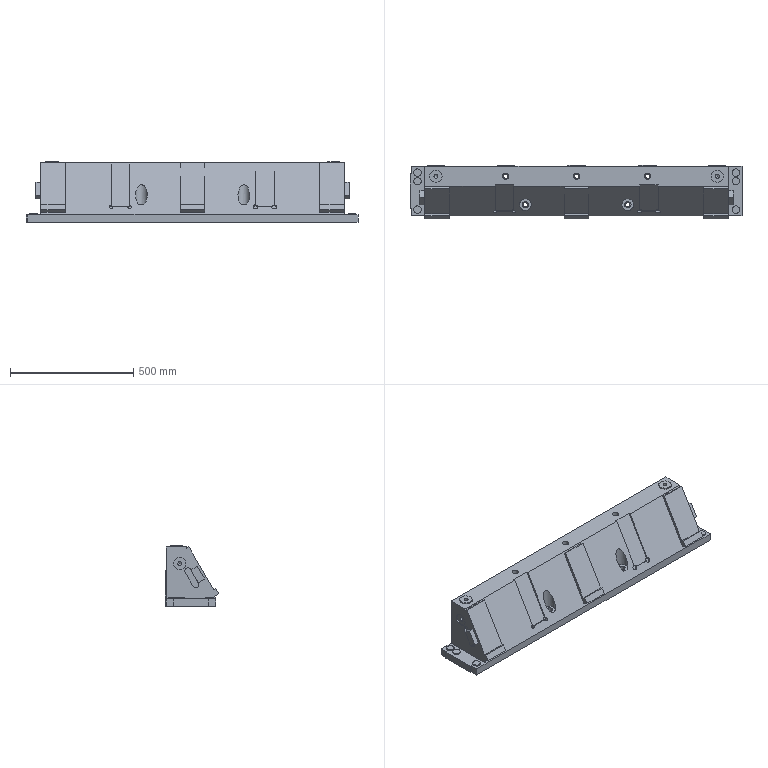Part | NX | features solid 2 | 1 solid | 163 faces | box 1345 x 217.346 x 245 mm | volume 34089938 mm3 | plane 123 | cylinder 36 | cone 4 | commonest cylinder face diameters 30 x6 17 x5 26 x5 16 x4 25 x4 50 x4